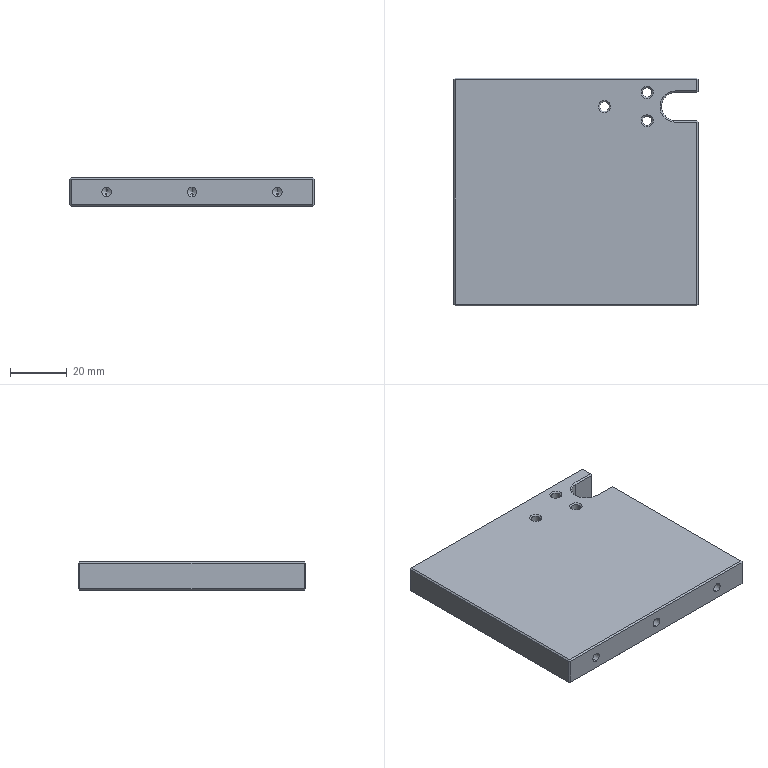Part | STEP file | Circlip fixture-upright plate | 1 solid | 93 faces | box 86 x 80 x 10 mm | volume 66708 mm3 | plane 41 | cone 33 | cylinder 19 | commonest cylinder face diameters 3.3 x18 10 x1